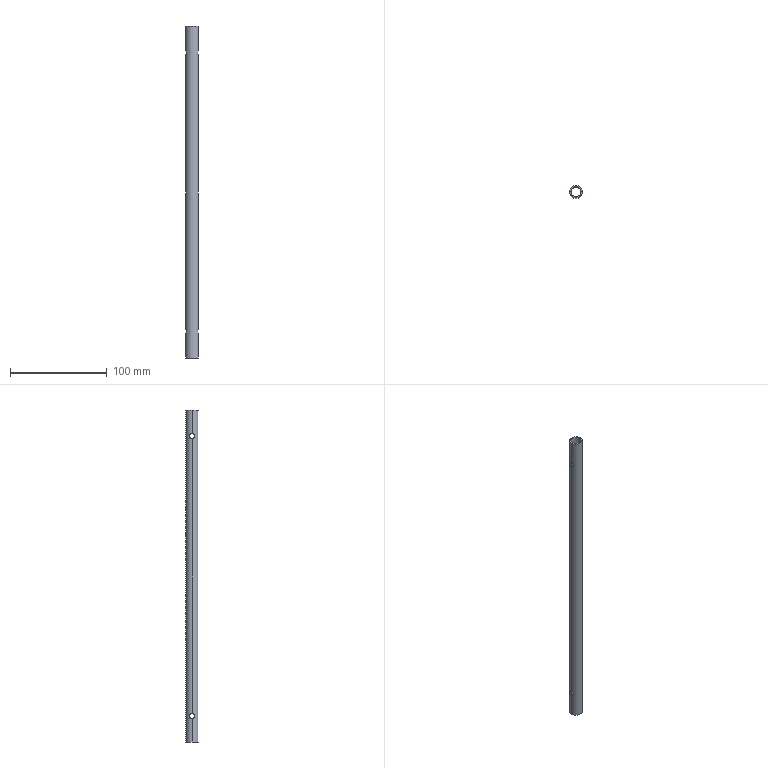Part | SolidWorks | features BaseBody 1 | 1 solid | 14 faces | box 13 x 13 x 343 mm | volume 15154 mm3 | cylinder 12 | plane 2 | commonest cylinder face diameters 5.2 x8 10.6 x2 13 x2
STEP:
#1=CARTESIAN_POINT('',(-6.5,0.,343.));
#2=VERTEX_POINT('',#1);
#3=CARTESIAN_POINT('',(6.5,0.,343.));
#4=VERTEX_POINT('',#3);
#5=CARTESIAN_POINT('',(0.,0.,343.));
#6=DIRECTION('',(0.,0.,-1.));
#7=DIRECTION('',(-1.,0.,0.));
#8=AXIS2_PLACEMENT_3D('',#5,#6,#7);
#9=CIRCLE('',#8,6.5);
#10=EDGE_CURVE('',#2,#4,#9,.T.);
#11=ORIENTED_EDGE('',*,*,#10,.T.);
#12=CARTESIAN_POINT('',(6.5,0.,318.6));
#13=VERTEX_POINT('',#12);
#14=CARTESIAN_POINT('',(6.5,0.,343.));
#15=DIRECTION('',(0.,0.,-1.));
#16=VECTOR('',#15,1000.);
#17=LINE('',#14,#16);
#18=EDGE_CURVE('',#4,#13,#17,.T.);
#19=ORIENTED_EDGE('',*,*,#18,.T.);
#20=CARTESIAN_POINT('',(6.5,0.,313.4));
#21=VERTEX_POINT('',#20);
#22=CARTESIAN_POINT('',(6.5,0.,318.6));
#23=CARTESIAN_POINT('',(6.5,0.1737,318.6));
#24=CARTESIAN_POINT('',(6.493,0.3441,318.583));
#25=CARTESIAN_POINT('',(6.467,0.6788,318.516));
#26=CARTESIAN_POINT('',(6.447,0.8449,318.465));
#27=CARTESIAN_POINT('',(6.398,1.159,318.334));
#28=CARTESIAN_POINT('',(6.369,1.308,318.254));
#29=CARTESIAN_POINT('',(6.304,1.589,318.065));
#30=CARTESIAN_POINT('',(6.269,1.72,317.957));
#31=CARTESIAN_POINT('',(6.165,2.076,317.601));
#32=CARTESIAN_POINT('',(6.093,2.269,317.314));
#33=CARTESIAN_POINT('',(6.015,2.464,316.847));
#34=CARTESIAN_POINT('',(5.994,2.515,316.681));
#35=CARTESIAN_POINT('',(5.965,2.583,316.345));
#36=CARTESIAN_POINT('',(5.957,2.6,316.175));
#37=CARTESIAN_POINT('',(5.957,2.6,315.832));
#38=CARTESIAN_POINT('',(5.965,2.583,315.658));
#39=CARTESIAN_POINT('',(5.993,2.516,315.323));
#40=CARTESIAN_POINT('',(6.014,2.466,315.159));
#41=CARTESIAN_POINT('',(6.067,2.335,314.843));
#42=CARTESIAN_POINT('',(6.097,2.254,314.694));
#43=CARTESIAN_POINT('',(6.163,2.067,314.414));
#44=CARTESIAN_POINT('',(6.199,1.959,314.282));
#45=CARTESIAN_POINT('',(6.269,1.721,314.044));
#46=CARTESIAN_POINT('',(6.304,1.592,313.937));
#47=CARTESIAN_POINT('',(6.368,1.311,313.748));
#48=CARTESIAN_POINT('',(6.398,1.16,313.667));
#49=CARTESIAN_POINT('',(6.471,0.6911,313.471));
#50=CARTESIAN_POINT('',(6.5,0.3472,313.4));
#51=CARTESIAN_POINT('',(6.5,0.,313.4));
#52=B_SPLINE_CURVE_WITH_KNOTS('',3,(#22,#23,#24,#25,#26,#27,#28,#29,#30,#31,#32,#33,#34,#35,#36,#37,#38,#39,#40,#41,#42,#43,#44,#45,#46,#47,#48,#49,#50,#51),.UNSPECIFIED.,.F.,.F.,(4,2,2,2,2,2,2,2,2,2,2,2,2,2,4),(0.008212,0.008725,0.009238,0.009751,0.01026,0.01129,0.0118,0.01232,0.01283,0.01334,0.01386,0.01437,0.01488,0.0154,0.01642),.UNSPECIFIED.);
#53=EDGE_CURVE('',#13,#21,#52,.T.);
#54=ORIENTED_EDGE('',*,*,#53,.T.);
#55=CARTESIAN_POINT('',(6.5,0.,29.6));
#56=VERTEX_POINT('',#55);
#57=CARTESIAN_POINT('',(6.5,0.,343.));
#58=DIRECTION('',(0.,0.,-1.));
#59=VECTOR('',#58,1000.);
#60=LINE('',#57,#59);
#61=EDGE_CURVE('',#21,#56,#60,.T.);
#62=ORIENTED_EDGE('',*,*,#61,.T.);
#63=CARTESIAN_POINT('',(6.5,0.,24.4));
#64=VERTEX_POINT('',#63);
#65=CARTESIAN_POINT('',(6.5,0.,29.6));
#66=CARTESIAN_POINT('',(6.5,0.1737,29.6));
#67=CARTESIAN_POINT('',(6.493,0.3441,29.583));
#68=CARTESIAN_POINT('',(6.467,0.6788,29.516));
#69=CARTESIAN_POINT('',(6.447,0.8449,29.465));
#70=CARTESIAN_POINT('',(6.398,1.159,29.334));
#71=CARTESIAN_POINT('',(6.369,1.308,29.254));
#72=CARTESIAN_POINT('',(6.304,1.589,29.065));
#73=CARTESIAN_POINT('',(6.269,1.72,28.957));
#74=CARTESIAN_POINT('',(6.165,2.076,28.601));
#75=CARTESIAN_POINT('',(6.093,2.269,28.314));
#76=CARTESIAN_POINT('',(6.015,2.464,27.847));
#77=CARTESIAN_POINT('',(5.994,2.515,27.681));
#78=CARTESIAN_POINT('',(5.965,2.583,27.345));
#79=CARTESIAN_POINT('',(5.957,2.6,27.175));
#80=CARTESIAN_POINT('',(5.957,2.6,26.832));
#81=CARTESIAN_POINT('',(5.965,2.583,26.658));
#82=CARTESIAN_POINT('',(5.993,2.516,26.323));
#83=CARTESIAN_POINT('',(6.014,2.466,26.159));
#84=CARTESIAN_POINT('',(6.067,2.335,25.843));
#85=CARTESIAN_POINT('',(6.097,2.254,25.694));
#86=CARTESIAN_POINT('',(6.163,2.067,25.414));
#87=CARTESIAN_POINT('',(6.199,1.959,25.282));
#88=CARTESIAN_POINT('',(6.269,1.721,25.044));
#89=CARTESIAN_POINT('',(6.304,1.592,24.937));
#90=CARTESIAN_POINT('',(6.368,1.311,24.748));
#91=CARTESIAN_POINT('',(6.398,1.16,24.667));
#92=CARTESIAN_POINT('',(6.471,0.6911,24.471));
#93=CARTESIAN_POINT('',(6.5,0.3472,24.4));
#94=CARTESIAN_POINT('',(6.5,0.,24.4));
#95=B_SPLINE_CURVE_WITH_KNOTS('',3,(#65,#66,#67,#68,#69,#70,#71,#72,#73,#74,#75,#76,#77,#78,#79,#80,#81,#82,#83,#84,#85,#86,#87,#88,#89,#90,#91,#92,#93,#94),.UNSPECIFIED.,.F.,.F.,(4,2,2,2,2,2,2,2,2,2,2,2,2,2,4),(0.008212,0.008725,0.009238,0.009751,0.01026,0.01129,0.0118,0.01232,0.01283,0.01334,0.01386,0.01437,0.01488,0.0154,0.01642),.UNSPECIFIED.);
#96=EDGE_CURVE('',#56,#64,#95,.T.);
#97=ORIENTED_EDGE('',*,*,#96,.T.);
#98=CARTESIAN_POINT('',(6.5,0.,0.));
#99=VERTEX_POINT('',#98);
#100=CARTESIAN_POINT('',(6.5,0.,343.));
#101=DIRECTION('',(0.,0.,-1.));
#102=VECTOR('',#101,1000.);
#103=LINE('',#100,#102);
#104=EDGE_CURVE('',#64,#99,#103,.T.);
#105=ORIENTED_EDGE('',*,*,#104,.T.);
#106=CARTESIAN_POINT('',(-6.5,0.,0.));
#107=VERTEX_POINT('',#106);
#108=CARTESIAN_POINT('',(0.,0.,0.));
#109=DIRECTION('',(0.,0.,1.));
#110=DIRECTION('',(-1.,0.,0.));
#111=AXIS2_PLACEMENT_3D('',#108,#109,#110);
#112=CIRCLE('',#111,6.5);
#113=EDGE_CURVE('',#99,#107,#112,.T.);
#114=ORIENTED_EDGE('',*,*,#113,.T.);
#115=CARTESIAN_POINT('',(-6.5,0.,24.4));
#116=VERTEX_POINT('',#115);
#117=CARTESIAN_POINT('',(-6.5,0.,343.));
#118=DIRECTION('',(0.,0.,-1.));
#119=VECTOR('',#118,1000.);
#120=LINE('',#117,#119);
#121=EDGE_CURVE('',#116,#107,#120,.T.);
#122=ORIENTED_EDGE('',*,*,#121,.F.);
#123=CARTESIAN_POINT('',(-6.5,0.,29.6));
#124=VERTEX_POINT('',#123);
#125=CARTESIAN_POINT('',(-6.5,0.,24.4));
#126=CARTESIAN_POINT('',(-6.5,0.1737,24.4));
#127=CARTESIAN_POINT('',(-6.493,0.3441,24.417));
#128=CARTESIAN_POINT('',(-6.467,0.6788,24.484));
#129=CARTESIAN_POINT('',(-6.447,0.8449,24.535));
#130=CARTESIAN_POINT('',(-6.398,1.159,24.666));
#131=CARTESIAN_POINT('',(-6.369,1.308,24.746));
#132=CARTESIAN_POINT('',(-6.304,1.589,24.935));
#133=CARTESIAN_POINT('',(-6.269,1.72,25.043));
#134=CARTESIAN_POINT('',(-6.165,2.076,25.399));
#135=CARTESIAN_POINT('',(-6.093,2.269,25.686));
#136=CARTESIAN_POINT('',(-6.015,2.464,26.153));
#137=CARTESIAN_POINT('',(-5.994,2.515,26.319));
#138=CARTESIAN_POINT('',(-5.965,2.583,26.655));
#139=CARTESIAN_POINT('',(-5.957,2.6,26.825));
#140=CARTESIAN_POINT('',(-5.957,2.6,27.168));
#141=CARTESIAN_POINT('',(-5.965,2.583,27.342));
#142=CARTESIAN_POINT('',(-5.993,2.516,27.677));
#143=CARTESIAN_POINT('',(-6.014,2.466,27.841));
#144=CARTESIAN_POINT('',(-6.067,2.335,28.157));
#145=CARTESIAN_POINT('',(-6.097,2.254,28.306));
#146=CARTESIAN_POINT('',(-6.163,2.067,28.586));
#147=CARTESIAN_POINT('',(-6.199,1.959,28.718));
#148=CARTESIAN_POINT('',(-6.269,1.721,28.956));
#149=CARTESIAN_POINT('',(-6.304,1.592,29.063));
#150=CARTESIAN_POINT('',(-6.368,1.311,29.252));
#151=CARTESIAN_POINT('',(-6.398,1.16,29.333));
#152=CARTESIAN_POINT('',(-6.471,0.6911,29.529));
#153=CARTESIAN_POINT('',(-6.5,0.3472,29.6));
#154=CARTESIAN_POINT('',(-6.5,0.,29.6));
#155=B_SPLINE_CURVE_WITH_KNOTS('',3,(#125,#126,#127,#128,#129,#130,#131,#132,#133,#134,#135,#136,#137,#138,#139,#140,#141,#142,#143,#144,#145,#146,#147,#148,#149,#150,#151,#152,#153,#154),.UNSPECIFIED.,.F.,.F.,(4,2,2,2,2,2,2,2,2,2,2,2,2,2,4),(0.008212,0.008725,0.009238,0.009751,0.01026,0.01129,0.0118,0.01232,0.01283,0.01334,0.01386,0.01437,0.01488,0.0154,0.01642),.UNSPECIFIED.);
#156=EDGE_CURVE('',#116,#124,#155,.T.);
#157=ORIENTED_EDGE('',*,*,#156,.T.);
#158=CARTESIAN_POINT('',(-6.5,0.,313.4));
#159=VERTEX_POINT('',#158);
#160=CARTESIAN_POINT('',(-6.5,0.,343.));
#161=DIRECTION('',(0.,0.,-1.));
#162=VECTOR('',#161,1000.);
#163=LINE('',#160,#162);
#164=EDGE_CURVE('',#159,#124,#163,.T.);
#165=ORIENTED_EDGE('',*,*,#164,.F.);
#166=CARTESIAN_POINT('',(-6.5,0.,318.6));
#167=VERTEX_POINT('',#166);
#168=CARTESIAN_POINT('',(-6.5,0.,313.4));
#169=CARTESIAN_POINT('',(-6.5,0.1737,313.4));
#170=CARTESIAN_POINT('',(-6.493,0.3441,313.417));
#171=CARTESIAN_POINT('',(-6.467,0.6788,313.484));
#172=CARTESIAN_POINT('',(-6.447,0.8449,313.535));
#173=CARTESIAN_POINT('',(-6.398,1.159,313.666));
#174=CARTESIAN_POINT('',(-6.369,1.308,313.746));
#175=CARTESIAN_POINT('',(-6.304,1.589,313.935));
#176=CARTESIAN_POINT('',(-6.269,1.72,314.043));
#177=CARTESIAN_POINT('',(-6.165,2.076,314.399));
#178=CARTESIAN_POINT('',(-6.093,2.269,314.686));
#179=CARTESIAN_POINT('',(-6.015,2.464,315.153));
#180=CARTESIAN_POINT('',(-5.994,2.515,315.319));
#181=CARTESIAN_POINT('',(-5.965,2.583,315.655));
#182=CARTESIAN_POINT('',(-5.957,2.6,315.825));
#183=CARTESIAN_POINT('',(-5.957,2.6,316.168));
#184=CARTESIAN_POINT('',(-5.965,2.583,316.342));
#185=CARTESIAN_POINT('',(-5.993,2.516,316.677));
#186=CARTESIAN_POINT('',(-6.014,2.466,316.841));
#187=CARTESIAN_POINT('',(-6.067,2.335,317.157));
#188=CARTESIAN_POINT('',(-6.097,2.254,317.306));
#189=CARTESIAN_POINT('',(-6.163,2.067,317.586));
#190=CARTESIAN_POINT('',(-6.199,1.959,317.718));
#191=CARTESIAN_POINT('',(-6.269,1.721,317.956));
#192=CARTESIAN_POINT('',(-6.304,1.592,318.063));
#193=CARTESIAN_POINT('',(-6.368,1.311,318.252));
#194=CARTESIAN_POINT('',(-6.398,1.16,318.333));
#195=CARTESIAN_POINT('',(-6.471,0.6911,318.529));
#196=CARTESIAN_POINT('',(-6.5,0.3472,318.6));
#197=CARTESIAN_POINT('',(-6.5,0.,318.6));
#198=B_SPLINE_CURVE_WITH_KNOTS('',3,(#168,#169,#170,#171,#172,#173,#174,#175,#176,#177,#178,#179,#180,#181,#182,#183,#184,#185,#186,#187,#188,#189,#190,#191,#192,#193,#194,#195,#196,#197),.UNSPECIFIED.,.F.,.F.,(4,2,2,2,2,2,2,2,2,2,2,2,2,2,4),(0.008212,0.008725,0.009238,0.009751,0.01026,0.01129,0.0118,0.01232,0.01283,0.01334,0.01386,0.01437,0.01488,0.0154,0.01642),.UNSPECIFIED.);
#199=EDGE_CURVE('',#159,#167,#198,.T.);
#200=ORIENTED_EDGE('',*,*,#199,.T.);
#201=CARTESIAN_POINT('',(-6.5,0.,343.));
#202=DIRECTION('',(0.,0.,-1.));
#203=VECTOR('',#202,1000.);
#204=LINE('',#201,#203);
#205=EDGE_CURVE('',#2,#167,#204,.T.);
#206=ORIENTED_EDGE('',*,*,#205,.F.);
#207=EDGE_LOOP('',(#11,#19,#54,#62,#97,#105,#114,#122,#157,#165,#200,#206));
#208=FACE_OUTER_BOUND('',#207,.T.);
#209=CARTESIAN_POINT('',(0.,0.,343.));
#210=DIRECTION('',(0.,0.,-1.));
#211=DIRECTION('',(-1.,0.,0.));
#212=AXIS2_PLACEMENT_3D('',#209,#210,#211);
#213=CYLINDRICAL_SURFACE('',#212,6.5);
#214=ADVANCED_FACE('',(#208),#213,.T.);
#215=CARTESIAN_POINT('',(5.3,0.,318.6));
#216=VERTEX_POINT('',#215);
#217=CARTESIAN_POINT('',(5.3,0.,313.4));
#218=VERTEX_POINT('',#217);
#219=CARTESIAN_POINT('',(5.3,0.,318.6));
#220=CARTESIAN_POINT('',(5.3,-0.1748,318.6));
#221=CARTESIAN_POINT('',(5.291,-0.3461,318.583));
#222=CARTESIAN_POINT('',(5.259,-0.6823,318.515));
#223=CARTESIAN_POINT('',(5.234,-0.8489,318.463));
#224=CARTESIAN_POINT('',(5.173,-1.163,318.332));
#225=CARTESIAN_POINT('',(5.137,-1.311,318.252));
#226=CARTESIAN_POINT('',(5.057,-1.592,318.063));
#227=CARTESIAN_POINT('',(5.014,-1.722,317.955));
#228=CARTESIAN_POINT('',(4.927,-1.958,317.719));
#229=CARTESIAN_POINT('',(4.882,-2.065,317.589));
#230=CARTESIAN_POINT('',(4.799,-2.253,317.309));
#231=CARTESIAN_POINT('',(4.76,-2.332,317.162));
#232=CARTESIAN_POINT('',(4.694,-2.463,316.85));
#233=CARTESIAN_POINT('',(4.666,-2.514,316.684));
#234=CARTESIAN_POINT('',(4.628,-2.582,316.348));
#235=CARTESIAN_POINT('',(4.619,-2.6,316.177));
#236=CARTESIAN_POINT('',(4.618,-2.6,315.832));
#237=CARTESIAN_POINT('',(4.628,-2.583,315.657));
#238=CARTESIAN_POINT('',(4.665,-2.515,315.32));
#239=CARTESIAN_POINT('',(4.693,-2.465,315.155));
#240=CARTESIAN_POINT('',(4.759,-2.333,314.84));
#241=CARTESIAN_POINT('',(4.798,-2.253,314.692));
#242=CARTESIAN_POINT('',(4.882,-2.066,314.413));
#243=CARTESIAN_POINT('',(4.926,-1.959,314.282));
#244=CARTESIAN_POINT('',(5.014,-1.723,314.046));
#245=CARTESIAN_POINT('',(5.057,-1.594,313.939));
#246=CARTESIAN_POINT('',(5.137,-1.313,313.749));
#247=CARTESIAN_POINT('',(5.173,-1.164,313.669));
#248=CARTESIAN_POINT('',(5.233,-0.8519,313.538));
#249=CARTESIAN_POINT('',(5.258,-0.6876,313.487));
#250=CARTESIAN_POINT('',(5.291,-0.3474,313.417));
#251=CARTESIAN_POINT('',(5.3,-0.1749,313.4));
#252=CARTESIAN_POINT('',(5.3,0.,313.4));
#253=B_SPLINE_CURVE_WITH_KNOTS('',3,(#219,#220,#221,#222,#223,#224,#225,#226,#227,#228,#229,#230,#231,#232,#233,#234,#235,#236,#237,#238,#239,#240,#241,#242,#243,#244,#245,#246,#247,#248,#249,#250,#251,#252),.UNSPECIFIED.,.F.,.F.,(4,2,2,2,2,2,2,2,2,2,2,2,2,2,2,2,4),(0.,0.0005163,0.001033,0.001549,0.002065,0.002581,0.003098,0.003614,0.00413,0.004646,0.005163,0.005679,0.006195,0.006712,0.007228,0.007744,0.00826),.UNSPECIFIED.);
#254=EDGE_CURVE('',#216,#218,#253,.T.);
#255=ORIENTED_EDGE('',*,*,#254,.F.);
#256=CARTESIAN_POINT('',(-6.5,0.,318.6));
#257=DIRECTION('',(1.,0.,0.));
#258=VECTOR('',#257,1000.);
#259=LINE('',#256,#258);
#260=EDGE_CURVE('',#216,#13,#259,.T.);
#261=ORIENTED_EDGE('',*,*,#260,.T.);
#262=CARTESIAN_POINT('',(6.5,0.,313.4));
#263=CARTESIAN_POINT('',(6.5,-0.1737,313.4));
#264=CARTESIAN_POINT('',(6.493,-0.3441,313.417));
#265=CARTESIAN_POINT('',(6.467,-0.6788,313.484));
#266=CARTESIAN_POINT('',(6.447,-0.8449,313.535));
#267=CARTESIAN_POINT('',(6.398,-1.159,313.666));
#268=CARTESIAN_POINT('',(6.369,-1.308,313.746));
#269=CARTESIAN_POINT('',(6.304,-1.589,313.935));
#270=CARTESIAN_POINT('',(6.269,-1.72,314.043));
#271=CARTESIAN_POINT('',(6.165,-2.076,314.399));
#272=CARTESIAN_POINT('',(6.093,-2.269,314.686));
#273=CARTESIAN_POINT('',(6.015,-2.464,315.153));
#274=CARTESIAN_POINT('',(5.994,-2.515,315.319));
#275=CARTESIAN_POINT('',(5.965,-2.583,315.655));
#276=CARTESIAN_POINT('',(5.957,-2.6,315.825));
#277=CARTESIAN_POINT('',(5.957,-2.6,316.168));
#278=CARTESIAN_POINT('',(5.965,-2.583,316.342));
#279=CARTESIAN_POINT('',(5.993,-2.516,316.677));
#280=CARTESIAN_POINT('',(6.014,-2.466,316.841));
#281=CARTESIAN_POINT('',(6.067,-2.335,317.157));
#282=CARTESIAN_POINT('',(6.097,-2.254,317.306));
#283=CARTESIAN_POINT('',(6.163,-2.067,317.586));
#284=CARTESIAN_POINT('',(6.199,-1.959,317.718));
#285=CARTESIAN_POINT('',(6.269,-1.721,317.956));
#286=CARTESIAN_POINT('',(6.304,-1.592,318.063));
#287=CARTESIAN_POINT('',(6.368,-1.311,318.252));
#288=CARTESIAN_POINT('',(6.398,-1.16,318.333));
#289=CARTESIAN_POINT('',(6.471,-0.6911,318.529));
#290=CARTESIAN_POINT('',(6.5,-0.3475,318.6));
#291=CARTESIAN_POINT('',(6.5,0.,318.6));
#292=B_SPLINE_CURVE_WITH_KNOTS('',3,(#262,#263,#264,#265,#266,#267,#268,#269,#270,#271,#272,#273,#274,#275,#276,#277,#278,#279,#280,#281,#282,#283,#284,#285,#286,#287,#288,#289,#290,#291),.UNSPECIFIED.,.F.,.F.,(4,2,2,2,2,2,2,2,2,2,2,2,2,2,4),(0.,0.0005133,0.001027,0.00154,0.002053,0.00308,0.003593,0.004106,0.004619,0.005133,0.005646,0.006159,0.006672,0.007186,0.008212),.UNSPECIFIED.);
#293=EDGE_CURVE('',#21,#13,#292,.T.);
#294=ORIENTED_EDGE('',*,*,#293,.F.);
#295=CARTESIAN_POINT('',(-6.5,0.,313.4));
#296=DIRECTION('',(1.,0.,0.));
#297=VECTOR('',#296,1000.);
#298=LINE('',#295,#297);
#299=EDGE_CURVE('',#218,#21,#298,.T.);
#300=ORIENTED_EDGE('',*,*,#299,.F.);
#301=EDGE_LOOP('',(#255,#261,#294,#300));
#302=FACE_OUTER_BOUND('',#301,.T.);
#303=CARTESIAN_POINT('',(-6.5,0.,316.));
#304=DIRECTION('',(1.,0.,0.));
#305=DIRECTION('',(0.,0.,-1.));
#306=AXIS2_PLACEMENT_3D('',#303,#304,#305);
#307=CYLINDRICAL_SURFACE('',#306,2.6);
#308=ADVANCED_FACE('',(#302),#307,.F.);
#309=CARTESIAN_POINT('',(5.3,0.,29.6));
#310=VERTEX_POINT('',#309);
#311=CARTESIAN_POINT('',(5.3,0.,24.4));
#312=VERTEX_POINT('',#311);
#313=CARTESIAN_POINT('',(5.3,0.,29.6));
#314=CARTESIAN_POINT('',(5.3,-0.1748,29.6));
#315=CARTESIAN_POINT('',(5.291,-0.3461,29.583));
#316=CARTESIAN_POINT('',(5.259,-0.6823,29.515));
#317=CARTESIAN_POINT('',(5.234,-0.8489,29.463));
#318=CARTESIAN_POINT('',(5.173,-1.163,29.332));
#319=CARTESIAN_POINT('',(5.137,-1.311,29.252));
#320=CARTESIAN_POINT('',(5.057,-1.592,29.063));
#321=CARTESIAN_POINT('',(5.014,-1.722,28.955));
#322=CARTESIAN_POINT('',(4.927,-1.958,28.719));
#323=CARTESIAN_POINT('',(4.882,-2.065,28.589));
#324=CARTESIAN_POINT('',(4.799,-2.253,28.309));
#325=CARTESIAN_POINT('',(4.76,-2.332,28.162));
#326=CARTESIAN_POINT('',(4.694,-2.463,27.85));
#327=CARTESIAN_POINT('',(4.666,-2.514,27.684));
#328=CARTESIAN_POINT('',(4.628,-2.582,27.348));
#329=CARTESIAN_POINT('',(4.619,-2.6,27.177));
#330=CARTESIAN_POINT('',(4.618,-2.6,26.832));
#331=CARTESIAN_POINT('',(4.628,-2.583,26.657));
#332=CARTESIAN_POINT('',(4.665,-2.515,26.32));
#333=CARTESIAN_POINT('',(4.693,-2.465,26.155));
#334=CARTESIAN_POINT('',(4.759,-2.333,25.84));
#335=CARTESIAN_POINT('',(4.798,-2.253,25.692));
#336=CARTESIAN_POINT('',(4.882,-2.066,25.413));
#337=CARTESIAN_POINT('',(4.926,-1.959,25.282));
#338=CARTESIAN_POINT('',(5.014,-1.723,25.046));
#339=CARTESIAN_POINT('',(5.057,-1.594,24.939));
#340=CARTESIAN_POINT('',(5.137,-1.313,24.749));
#341=CARTESIAN_POINT('',(5.173,-1.164,24.669));
#342=CARTESIAN_POINT('',(5.233,-0.8519,24.538));
#343=CARTESIAN_POINT('',(5.258,-0.6876,24.487));
#344=CARTESIAN_POINT('',(5.291,-0.3474,24.417));
#345=CARTESIAN_POINT('',(5.3,-0.1749,24.4));
#346=CARTESIAN_POINT('',(5.3,0.,24.4));
#347=B_SPLINE_CURVE_WITH_KNOTS('',3,(#313,#314,#315,#316,#317,#318,#319,#320,#321,#322,#323,#324,#325,#326,#327,#328,#329,#330,#331,#332,#333,#334,#335,#336,#337,#338,#339,#340,#341,#342,#343,#344,#345,#346),.UNSPECIFIED.,.F.,.F.,(4,2,2,2,2,2,2,2,2,2,2,2,2,2,2,2,4),(0.,0.0005163,0.001033,0.001549,0.002065,0.002581,0.003098,0.003614,0.00413,0.004646,0.005163,0.005679,0.006195,0.006712,0.007228,0.007744,0.00826),.UNSPECIFIED.);
#348=EDGE_CURVE('',#310,#312,#347,.T.);
#349=ORIENTED_EDGE('',*,*,#348,.F.);
#350=CARTESIAN_POINT('',(-6.5,0.,29.6));
#351=DIRECTION('',(1.,0.,0.));
#352=VECTOR('',#351,1000.);
#353=LINE('',#350,#352);
#354=EDGE_CURVE('',#310,#56,#353,.T.);
#355=ORIENTED_EDGE('',*,*,#354,.T.);
#356=CARTESIAN_POINT('',(6.5,0.,24.4));
#357=CARTESIAN_POINT('',(6.5,-0.1737,24.4));
#358=CARTESIAN_POINT('',(6.493,-0.3441,24.417));
#359=CARTESIAN_POINT('',(6.467,-0.6788,24.484));
#360=CARTESIAN_POINT('',(6.447,-0.8449,24.535));
#361=CARTESIAN_POINT('',(6.398,-1.159,24.666));
#362=CARTESIAN_POINT('',(6.369,-1.308,24.746));
#363=CARTESIAN_POINT('',(6.304,-1.589,24.935));
#364=CARTESIAN_POINT('',(6.269,-1.72,25.043));
#365=CARTESIAN_POINT('',(6.165,-2.076,25.399));
#366=CARTESIAN_POINT('',(6.093,-2.269,25.686));
#367=CARTESIAN_POINT('',(6.015,-2.464,26.153));
#368=CARTESIAN_POINT('',(5.994,-2.515,26.319));
#369=CARTESIAN_POINT('',(5.965,-2.583,26.655));
#370=CARTESIAN_POINT('',(5.957,-2.6,26.825));
#371=CARTESIAN_POINT('',(5.957,-2.6,27.168));
#372=CARTESIAN_POINT('',(5.965,-2.583,27.342));
#373=CARTESIAN_POINT('',(5.993,-2.516,27.677));
#374=CARTESIAN_POINT('',(6.014,-2.466,27.841));
#375=CARTESIAN_POINT('',(6.067,-2.335,28.157));
#376=CARTESIAN_POINT('',(6.097,-2.254,28.306));
#377=CARTESIAN_POINT('',(6.163,-2.067,28.586));
#378=CARTESIAN_POINT('',(6.199,-1.959,28.718));
#379=CARTESIAN_POINT('',(6.269,-1.721,28.956));
#380=CARTESIAN_POINT('',(6.304,-1.592,29.063));
#381=CARTESIAN_POINT('',(6.368,-1.311,29.252));
#382=CARTESIAN_POINT('',(6.398,-1.16,29.333));
#383=CARTESIAN_POINT('',(6.471,-0.6911,29.529));
#384=CARTESIAN_POINT('',(6.5,-0.3475,29.6));
#385=CARTESIAN_POINT('',(6.5,0.,29.6));
#386=B_SPLINE_CURVE_WITH_KNOTS('',3,(#356,#357,#358,#359,#360,#361,#362,#363,#364,#365,#366,#367,#368,#369,#370,#371,#372,#373,#374,#375,#376,#377,#378,#379,#380,#381,#382,#383,#384,#385),.UNSPECIFIED.,.F.,.F.,(4,2,2,2,2,2,2,2,2,2,2,2,2,2,4),(0.,0.0005133,0.001027,0.00154,0.002053,0.00308,0.003593,0.004106,0.004619,0.005133,0.005646,0.006159,0.006672,0.007186,0.008212),.UNSPECIFIED.);
#387=EDGE_CURVE('',#64,#56,#386,.T.);
#388=ORIENTED_EDGE('',*,*,#387,.F.);
#389=CARTESIAN_POINT('',(-6.5,0.,24.4));
#390=DIRECTION('',(1.,0.,0.));
#391=VECTOR('',#390,1000.);
#392=LINE('',#389,#391);
#393=EDGE_CURVE('',#312,#64,#392,.T.);
#394=ORIENTED_EDGE('',*,*,#393,.F.);
#395=EDGE_LOOP('',(#349,#355,#388,#394));
#396=FACE_OUTER_BOUND('',#395,.T.);
#397=CARTESIAN_POINT('',(-6.5,0.,27.));
#398=DIRECTION('',(1.,0.,0.));
#399=DIRECTION('',(0.,0.,-1.));
#400=AXIS2_PLACEMENT_3D('',#397,#398,#399);
#401=CYLINDRICAL_SURFACE('',#400,2.6);
#402=ADVANCED_FACE('',(#396),#401,.F.);
#403=CARTESIAN_POINT('',(-6.5,0.,29.6));
#404=CARTESIAN_POINT('',(-6.5,-0.1737,29.6));
#405=CARTESIAN_POINT('',(-6.493,-0.3441,29.583));
#406=CARTESIAN_POINT('',(-6.467,-0.6788,29.516));
#407=CARTESIAN_POINT('',(-6.447,-0.8449,29.465));
#408=CARTESIAN_POINT('',(-6.398,-1.159,29.334));
#409=CARTESIAN_POINT('',(-6.369,-1.308,29.254));
#410=CARTESIAN_POINT('',(-6.304,-1.589,29.065));
#411=CARTESIAN_POINT('',(-6.269,-1.72,28.957));
#412=CARTESIAN_POINT('',(-6.165,-2.076,28.601));
#413=CARTESIAN_POINT('',(-6.093,-2.269,28.314));
#414=CARTESIAN_POINT('',(-6.015,-2.464,27.847));
#415=CARTESIAN_POINT('',(-5.994,-2.515,27.681));
#416=CARTESIAN_POINT('',(-5.965,-2.583,27.345));
#417=CARTESIAN_POINT('',(-5.957,-2.6,27.175));
#418=CARTESIAN_POINT('',(-5.957,-2.6,26.832));
#419=CARTESIAN_POINT('',(-5.965,-2.583,26.658));
#420=CARTESIAN_POINT('',(-5.993,-2.516,26.323));
#421=CARTESIAN_POINT('',(-6.014,-2.466,26.159));
#422=CARTESIAN_POINT('',(-6.067,-2.335,25.843));
#423=CARTESIAN_POINT('',(-6.097,-2.254,25.694));
#424=CARTESIAN_POINT('',(-6.163,-2.067,25.414));
#425=CARTESIAN_POINT('',(-6.199,-1.959,25.282));
#426=CARTESIAN_POINT('',(-6.269,-1.721,25.044));
#427=CARTESIAN_POINT('',(-6.304,-1.592,24.937));
#428=CARTESIAN_POINT('',(-6.368,-1.311,24.748));
#429=CARTESIAN_POINT('',(-6.398,-1.16,24.667));
#430=CARTESIAN_POINT('',(-6.471,-0.6911,24.471));
#431=CARTESIAN_POINT('',(-6.5,-0.3475,24.4));
#432=CARTESIAN_POINT('',(-6.5,0.,24.4));
#433=B_SPLINE_CURVE_WITH_KNOTS('',3,(#403,#404,#405,#406,#407,#408,#409,#410,#411,#412,#413,#414,#415,#416,#417,#418,#419,#420,#421,#422,#423,#424,#425,#426,#427,#428,#429,#430,#431,#432),.UNSPECIFIED.,.F.,.F.,(4,2,2,2,2,2,2,2,2,2,2,2,2,2,4),(0.,0.0005133,0.001027,0.00154,0.002053,0.00308,0.003593,0.004106,0.004619,0.005133,0.005646,0.006159,0.006672,0.007186,0.008212),.UNSPECIFIED.);
#434=EDGE_CURVE('',#124,#116,#433,.T.);
#435=ORIENTED_EDGE('',*,*,#434,.F.);
#436=CARTESIAN_POINT('',(-5.3,0.,29.6));
#437=VERTEX_POINT('',#436);
#438=CARTESIAN_POINT('',(-6.5,0.,29.6));
#439=DIRECTION('',(1.,0.,0.));
#440=VECTOR('',#439,1000.);
#441=LINE('',#438,#440);
#442=EDGE_CURVE('',#124,#437,#441,.T.);
#443=ORIENTED_EDGE('',*,*,#442,.T.);
#444=CARTESIAN_POINT('',(-5.3,0.,24.4));
#445=VERTEX_POINT('',#444);
#446=CARTESIAN_POINT('',(-5.3,0.,24.4));
#447=CARTESIAN_POINT('',(-5.3,-0.1748,24.4));
#448=CARTESIAN_POINT('',(-5.291,-0.3461,24.417));
#449=CARTESIAN_POINT('',(-5.259,-0.6823,24.485));
#450=CARTESIAN_POINT('',(-5.234,-0.8489,24.537));
#451=CARTESIAN_POINT('',(-5.173,-1.163,24.668));
#452=CARTESIAN_POINT('',(-5.137,-1.311,24.748));
#453=CARTESIAN_POINT('',(-5.057,-1.592,24.937));
#454=CARTESIAN_POINT('',(-5.014,-1.722,25.045));
#455=CARTESIAN_POINT('',(-4.927,-1.958,25.281));
#456=CARTESIAN_POINT('',(-4.882,-2.065,25.411));
#457=CARTESIAN_POINT('',(-4.799,-2.253,25.691));
#458=CARTESIAN_POINT('',(-4.76,-2.332,25.838));
#459=CARTESIAN_POINT('',(-4.694,-2.463,26.15));
#460=CARTESIAN_POINT('',(-4.666,-2.514,26.316));
#461=CARTESIAN_POINT('',(-4.628,-2.582,26.652));
#462=CARTESIAN_POINT('',(-4.619,-2.6,26.823));
#463=CARTESIAN_POINT('',(-4.618,-2.6,27.168));
#464=CARTESIAN_POINT('',(-4.628,-2.583,27.343));
#465=CARTESIAN_POINT('',(-4.665,-2.515,27.68));
#466=CARTESIAN_POINT('',(-4.693,-2.465,27.845));
#467=CARTESIAN_POINT('',(-4.759,-2.333,28.16));
#468=CARTESIAN_POINT('',(-4.798,-2.253,28.308));
#469=CARTESIAN_POINT('',(-4.882,-2.066,28.587));
#470=CARTESIAN_POINT('',(-4.926,-1.959,28.718));
#471=CARTESIAN_POINT('',(-5.014,-1.723,28.954));
#472=CARTESIAN_POINT('',(-5.057,-1.594,29.061));
#473=CARTESIAN_POINT('',(-5.137,-1.313,29.251));
#474=CARTESIAN_POINT('',(-5.173,-1.164,29.331));
#475=CARTESIAN_POINT('',(-5.233,-0.8519,29.462));
#476=CARTESIAN_POINT('',(-5.258,-0.6876,29.513));
#477=CARTESIAN_POINT('',(-5.291,-0.3474,29.583));
#478=CARTESIAN_POINT('',(-5.3,-0.1749,29.6));
#479=CARTESIAN_POINT('',(-5.3,0.,29.6));
#480=B_SPLINE_CURVE_WITH_KNOTS('',3,(#446,#447,#448,#449,#450,#451,#452,#453,#454,#455,#456,#457,#458,#459,#460,#461,#462,#463,#464,#465,#466,#467,#468,#469,#470,#471,#472,#473,#474,#475,#476,#477,#478,#479),.UNSPECIFIED.,.F.,.F.,(4,2,2,2,2,2,2,2,2,2,2,2,2,2,2,2,4),(0.,0.0005163,0.001033,0.001549,0.002065,0.002581,0.003098,0.003614,0.00413,0.004646,0.005163,0.005679,0.006195,0.006712,0.007228,0.007744,0.00826),.UNSPECIFIED.);
#481=EDGE_CURVE('',#445,#437,#480,.T.);
#482=ORIENTED_EDGE('',*,*,#481,.F.);
#483=CARTESIAN_POINT('',(-6.5,0.,24.4));
#484=DIRECTION('',(1.,0.,0.));
#485=VECTOR('',#484,1000.);
#486=LINE('',#483,#485);
#487=EDGE_CURVE('',#116,#445,#486,.T.);
#488=ORIENTED_EDGE('',*,*,#487,.F.);
#489=EDGE_LOOP('',(#435,#443,#482,#488));
#490=FACE_OUTER_BOUND('',#489,.T.);
#491=CARTESIAN_POINT('',(-6.5,0.,27.));
#492=DIRECTION('',(1.,0.,0.));
#493=DIRECTION('',(0.,0.,-1.));
#494=AXIS2_PLACEMENT_3D('',#491,#492,#493);
#495=CYLINDRICAL_SURFACE('',#494,2.6);
#496=ADVANCED_FACE('',(#490),#495,.F.);
#497=CARTESIAN_POINT('',(-6.5,0.,318.6));
#498=CARTESIAN_POINT('',(-6.5,-0.1737,318.6));
#499=CARTESIAN_POINT('',(-6.493,-0.3441,318.583));
#500=CARTESIAN_POINT('',(-6.467,-0.6788,318.516));
#501=CARTESIAN_POINT('',(-6.447,-0.8449,318.465));
#502=CARTESIAN_POINT('',(-6.398,-1.159,318.334));
#503=CARTESIAN_POINT('',(-6.369,-1.308,318.254));
#504=CARTESIAN_POINT('',(-6.304,-1.589,318.065));
#505=CARTESIAN_POINT('',(-6.269,-1.72,317.957));
#506=CARTESIAN_POINT('',(-6.165,-2.076,317.601));
#507=CARTESIAN_POINT('',(-6.093,-2.269,317.314));
#508=CARTESIAN_POINT('',(-6.015,-2.464,316.847));
#509=CARTESIAN_POINT('',(-5.994,-2.515,316.681));
#510=CARTESIAN_POINT('',(-5.965,-2.583,316.345));
#511=CARTESIAN_POINT('',(-5.957,-2.6,316.175));
#512=CARTESIAN_POINT('',(-5.957,-2.6,315.832));
#513=CARTESIAN_POINT('',(-5.965,-2.583,315.658));
#514=CARTESIAN_POINT('',(-5.993,-2.516,315.323));
#515=CARTESIAN_POINT('',(-6.014,-2.466,315.159));
#516=CARTESIAN_POINT('',(-6.067,-2.335,314.843));
#517=CARTESIAN_POINT('',(-6.097,-2.254,314.694));
#518=CARTESIAN_POINT('',(-6.163,-2.067,314.414));
#519=CARTESIAN_POINT('',(-6.199,-1.959,314.282));
#520=CARTESIAN_POINT('',(-6.269,-1.721,314.044));
#521=CARTESIAN_POINT('',(-6.304,-1.592,313.937));
#522=CARTESIAN_POINT('',(-6.368,-1.311,313.748));
#523=CARTESIAN_POINT('',(-6.398,-1.16,313.667));
#524=CARTESIAN_POINT('',(-6.471,-0.6911,313.471));
#525=CARTESIAN_POINT('',(-6.5,-0.3475,313.4));
#526=CARTESIAN_POINT('',(-6.5,0.,313.4));
#527=B_SPLINE_CURVE_WITH_KNOTS('',3,(#497,#498,#499,#500,#501,#502,#503,#504,#505,#506,#507,#508,#509,#510,#511,#512,#513,#514,#515,#516,#517,#518,#519,#520,#521,#522,#523,#524,#525,#526),.UNSPECIFIED.,.F.,.F.,(4,2,2,2,2,2,2,2,2,2,2,2,2,2,4),(0.,0.0005133,0.001027,0.00154,0.002053,0.00308,0.003593,0.004106,0.004619,0.005133,0.005646,0.006159,0.006672,0.007186,0.008212),.UNSPECIFIED.);
#528=EDGE_CURVE('',#167,#159,#527,.T.);
#529=ORIENTED_EDGE('',*,*,#528,.F.);
#530=CARTESIAN_POINT('',(-5.3,0.,318.6));
#531=VERTEX_POINT('',#530);
#532=CARTESIAN_POINT('',(-6.5,0.,318.6));
#533=DIRECTION('',(1.,0.,0.));
#534=VECTOR('',#533,1000.);
#535=LINE('',#532,#534);
#536=EDGE_CURVE('',#167,#531,#535,.T.);
#537=ORIENTED_EDGE('',*,*,#536,.T.);
#538=CARTESIAN_POINT('',(-5.3,0.,313.4));
#539=VERTEX_POINT('',#538);
#540=CARTESIAN_POINT('',(-5.3,0.,313.4));
#541=CARTESIAN_POINT('',(-5.3,-0.1748,313.4));
#542=CARTESIAN_POINT('',(-5.291,-0.3461,313.417));
#543=CARTESIAN_POINT('',(-5.259,-0.6823,313.485));
#544=CARTESIAN_POINT('',(-5.234,-0.8489,313.537));
#545=CARTESIAN_POINT('',(-5.173,-1.163,313.668));
#546=CARTESIAN_POINT('',(-5.137,-1.311,313.748));
#547=CARTESIAN_POINT('',(-5.057,-1.592,313.937));
#548=CARTESIAN_POINT('',(-5.014,-1.722,314.045));
#549=CARTESIAN_POINT('',(-4.927,-1.958,314.281));
#550=CARTESIAN_POINT('',(-4.882,-2.065,314.411));
#551=CARTESIAN_POINT('',(-4.799,-2.253,314.691));
#552=CARTESIAN_POINT('',(-4.76,-2.332,314.838));
#553=CARTESIAN_POINT('',(-4.694,-2.463,315.15));
#554=CARTESIAN_POINT('',(-4.666,-2.514,315.316));
#555=CARTESIAN_POINT('',(-4.628,-2.582,315.652));
#556=CARTESIAN_POINT('',(-4.619,-2.6,315.823));
#557=CARTESIAN_POINT('',(-4.618,-2.6,316.168));
#558=CARTESIAN_POINT('',(-4.628,-2.583,316.343));
#559=CARTESIAN_POINT('',(-4.665,-2.515,316.68));
#560=CARTESIAN_POINT('',(-4.693,-2.465,316.845));
#561=CARTESIAN_POINT('',(-4.759,-2.333,317.16));
#562=CARTESIAN_POINT('',(-4.798,-2.253,317.308));
#563=CARTESIAN_POINT('',(-4.882,-2.066,317.587));
#564=CARTESIAN_POINT('',(-4.926,-1.959,317.718));
#565=CARTESIAN_POINT('',(-5.014,-1.723,317.954));
#566=CARTESIAN_POINT('',(-5.057,-1.594,318.061));
#567=CARTESIAN_POINT('',(-5.137,-1.313,318.251));
#568=CARTESIAN_POINT('',(-5.173,-1.164,318.331));
#569=CARTESIAN_POINT('',(-5.233,-0.8519,318.462));
#570=CARTESIAN_POINT('',(-5.258,-0.6876,318.513));
#571=CARTESIAN_POINT('',(-5.291,-0.3474,318.583));
#572=CARTESIAN_POINT('',(-5.3,-0.1749,318.6));
#573=CARTESIAN_POINT('',(-5.3,0.,318.6));
#574=B_SPLINE_CURVE_WITH_KNOTS('',3,(#540,#541,#542,#543,#544,#545,#546,#547,#548,#549,#550,#551,#552,#553,#554,#555,#556,#557,#558,#559,#560,#561,#562,#563,#564,#565,#566,#567,#568,#569,#570,#571,#572,#573),.UNSPECIFIED.,.F.,.F.,(4,2,2,2,2,2,2,2,2,2,2,2,2,2,2,2,4),(0.,0.0005163,0.001033,0.001549,0.002065,0.002581,0.003098,0.003614,0.00413,0.004646,0.005163,0.005679,0.006195,0.006712,0.007228,0.007744,0.00826),.UNSPECIFIED.);
#575=EDGE_CURVE('',#539,#531,#574,.T.);
#576=ORIENTED_EDGE('',*,*,#575,.F.);
#577=CARTESIAN_POINT('',(-6.5,0.,313.4));
#578=DIRECTION('',(1.,0.,0.));
#579=VECTOR('',#578,1000.);
#580=LINE('',#577,#579);
#581=EDGE_CURVE('',#159,#539,#580,.T.);
#582=ORIENTED_EDGE('',*,*,#581,.F.);
#583=EDGE_LOOP('',(#529,#537,#576,#582));
#584=FACE_OUTER_BOUND('',#583,.T.);
#585=CARTESIAN_POINT('',(-6.5,0.,316.));
#586=DIRECTION('',(1.,0.,0.));
#587=DIRECTION('',(0.,0.,-1.));
#588=AXIS2_PLACEMENT_3D('',#585,#586,#587);
#589=CYLINDRICAL_SURFACE('',#588,2.6);
#590=ADVANCED_FACE('',(#584),#589,.F.);
#591=CARTESIAN_POINT('',(5.3,0.,343.));
#592=VERTEX_POINT('',#591);
#593=CARTESIAN_POINT('',(-5.3,0.,343.));
#594=VERTEX_POINT('',#593);
#595=CARTESIAN_POINT('',(0.,0.,343.));
#596=DIRECTION('',(0.,0.,-1.));
#597=DIRECTION('',(-1.,0.,0.));
#598=AXIS2_PLACEMENT_3D('',#595,#596,#597);
#599=CIRCLE('',#598,5.3);
#600=EDGE_CURVE('',#592,#594,#599,.T.);
#601=ORIENTED_EDGE('',*,*,#600,.F.);
#602=CARTESIAN_POINT('',(5.3,0.,343.));
#603=DIRECTION('',(0.,0.,-1.));
#604=VECTOR('',#603,1000.);
#605=LINE('',#602,#604);
#606=EDGE_CURVE('',#592,#216,#605,.T.);
#607=ORIENTED_EDGE('',*,*,#606,.T.);
#608=ORIENTED_EDGE('',*,*,#254,.T.);
#609=CARTESIAN_POINT('',(5.3,0.,343.));
#610=DIRECTION('',(0.,0.,-1.));
#611=VECTOR('',#610,1000.);
#612=LINE('',#609,#611);
#613=EDGE_CURVE('',#218,#310,#612,.T.);
#614=ORIENTED_EDGE('',*,*,#613,.T.);
#615=ORIENTED_EDGE('',*,*,#348,.T.);
#616=CARTESIAN_POINT('',(5.3,0.,0.));
#617=VERTEX_POINT('',#616);
#618=CARTESIAN_POINT('',(5.3,0.,343.));
#619=DIRECTION('',(0.,0.,-1.));
#620=VECTOR('',#619,1000.);
#621=LINE('',#618,#620);
#622=EDGE_CURVE('',#312,#617,#621,.T.);
#623=ORIENTED_EDGE('',*,*,#622,.T.);
#624=CARTESIAN_POINT('',(-5.3,0.,0.));
#625=VERTEX_POINT('',#624);
#626=CARTESIAN_POINT('',(0.,0.,0.));
#627=DIRECTION('',(0.,0.,-1.));
#628=DIRECTION('',(-1.,0.,0.));
#629=AXIS2_PLACEMENT_3D('',#626,#627,#628);
#630=CIRCLE('',#629,5.3);
#631=EDGE_CURVE('',#617,#625,#630,.T.);
#632=ORIENTED_EDGE('',*,*,#631,.T.);
#633=CARTESIAN_POINT('',(-5.3,0.,343.));
#634=DIRECTION('',(0.,0.,-1.));
#635=VECTOR('',#634,1000.);
#636=LINE('',#633,#635);
#637=EDGE_CURVE('',#445,#625,#636,.T.);
#638=ORIENTED_EDGE('',*,*,#637,.F.);
#639=ORIENTED_EDGE('',*,*,#481,.T.);
#640=CARTESIAN_POINT('',(-5.3,0.,343.));
#641=DIRECTION('',(0.,0.,-1.));
#642=VECTOR('',#641,1000.);
#643=LINE('',#640,#642);
#644=EDGE_CURVE('',#539,#437,#643,.T.);
#645=ORIENTED_EDGE('',*,*,#644,.F.);
#646=ORIENTED_EDGE('',*,*,#575,.T.);
#647=CARTESIAN_POINT('',(-5.3,0.,343.));
#648=DIRECTION('',(0.,0.,-1.));
#649=VECTOR('',#648,1000.);
#650=LINE('',#647,#649);
#651=EDGE_CURVE('',#594,#531,#650,.T.);
#652=ORIENTED_EDGE('',*,*,#651,.F.);
#653=EDGE_LOOP('',(#601,#607,#608,#614,#615,#623,#632,#638,#639,#645,#646,#652));
#654=FACE_OUTER_BOUND('',#653,.T.);
#655=CARTESIAN_POINT('',(0.,0.,343.));
#656=DIRECTION('',(0.,0.,-1.));
#657=DIRECTION('',(-1.,0.,0.));
#658=AXIS2_PLACEMENT_3D('',#655,#656,#657);
#659=CYLINDRICAL_SURFACE('',#658,5.3);
#660=ADVANCED_FACE('',(#654),#659,.F.);
#661=ORIENTED_EDGE('',*,*,#18,.F.);
#662=CARTESIAN_POINT('',(0.,0.,343.));
#663=DIRECTION('',(0.,0.,-1.));
#664=DIRECTION('',(-1.,0.,0.));
#665=AXIS2_PLACEMENT_3D('',#662,#663,#664);
#666=CIRCLE('',#665,6.5);
#667=EDGE_CURVE('',#4,#2,#666,.T.);
#668=ORIENTED_EDGE('',*,*,#667,.T.);
#669=ORIENTED_EDGE('',*,*,#205,.T.);
#670=ORIENTED_EDGE('',*,*,#528,.T.);
#671=ORIENTED_EDGE('',*,*,#164,.T.);
#672=ORIENTED_EDGE('',*,*,#434,.T.);
#673=ORIENTED_EDGE('',*,*,#121,.T.);
#674=CARTESIAN_POINT('',(0.,0.,0.));
#675=DIRECTION('',(0.,0.,1.));
#676=DIRECTION('',(-1.,0.,0.));
#677=AXIS2_PLACEMENT_3D('',#674,#675,#676);
#678=CIRCLE('',#677,6.5);
#679=EDGE_CURVE('',#107,#99,#678,.T.);
#680=ORIENTED_EDGE('',*,*,#679,.T.);
#681=ORIENTED_EDGE('',*,*,#104,.F.);
#682=ORIENTED_EDGE('',*,*,#387,.T.);
#683=ORIENTED_EDGE('',*,*,#61,.F.);
#684=ORIENTED_EDGE('',*,*,#293,.T.);
#685=EDGE_LOOP('',(#661,#668,#669,#670,#671,#672,#673,#680,#681,#682,#683,#684));
#686=FACE_OUTER_BOUND('',#685,.T.);
#687=CARTESIAN_POINT('',(0.,0.,343.));
#688=DIRECTION('',(0.,0.,-1.));
#689=DIRECTION('',(-1.,0.,0.));
#690=AXIS2_PLACEMENT_3D('',#687,#688,#689);
#691=CYLINDRICAL_SURFACE('',#690,6.5);
#692=ADVANCED_FACE('',(#686),#691,.T.);
#693=ORIENTED_EDGE('',*,*,#260,.F.);
#694=CARTESIAN_POINT('',(5.3,0.,313.4));
#695=CARTESIAN_POINT('',(5.3,0.1748,313.4));
#696=CARTESIAN_POINT('',(5.291,0.3461,313.417));
#697=CARTESIAN_POINT('',(5.259,0.6823,313.485));
#698=CARTESIAN_POINT('',(5.234,0.8489,313.537));
#699=CARTESIAN_POINT('',(5.173,1.163,313.668));
#700=CARTESIAN_POINT('',(5.137,1.311,313.748));
#701=CARTESIAN_POINT('',(5.057,1.592,313.937));
#702=CARTESIAN_POINT('',(5.014,1.722,314.045));
#703=CARTESIAN_POINT('',(4.927,1.958,314.281));
#704=CARTESIAN_POINT('',(4.882,2.065,314.411));
#705=CARTESIAN_POINT('',(4.799,2.253,314.691));
#706=CARTESIAN_POINT('',(4.76,2.332,314.838));
#707=CARTESIAN_POINT('',(4.694,2.463,315.15));
#708=CARTESIAN_POINT('',(4.666,2.514,315.316));
#709=CARTESIAN_POINT('',(4.628,2.582,315.652));
#710=CARTESIAN_POINT('',(4.619,2.6,315.823));
#711=CARTESIAN_POINT('',(4.618,2.6,316.168));
#712=CARTESIAN_POINT('',(4.628,2.583,316.343));
#713=CARTESIAN_POINT('',(4.665,2.515,316.68));
#714=CARTESIAN_POINT('',(4.693,2.465,316.845));
#715=CARTESIAN_POINT('',(4.759,2.333,317.16));
#716=CARTESIAN_POINT('',(4.798,2.253,317.308));
#717=CARTESIAN_POINT('',(4.882,2.066,317.587));
#718=CARTESIAN_POINT('',(4.926,1.959,317.718));
#719=CARTESIAN_POINT('',(5.014,1.723,317.954));
#720=CARTESIAN_POINT('',(5.057,1.594,318.061));
#721=CARTESIAN_POINT('',(5.137,1.313,318.251));
#722=CARTESIAN_POINT('',(5.173,1.164,318.331));
#723=CARTESIAN_POINT('',(5.264,0.696,318.528));
#724=CARTESIAN_POINT('',(5.3,0.3492,318.6));
#725=CARTESIAN_POINT('',(5.3,0.,318.6));
#726=B_SPLINE_CURVE_WITH_KNOTS('',3,(#694,#695,#696,#697,#698,#699,#700,#701,#702,#703,#704,#705,#706,#707,#708,#709,#710,#711,#712,#713,#714,#715,#716,#717,#718,#719,#720,#721,#722,#723,#724,#725),.UNSPECIFIED.,.F.,.F.,(4,2,2,2,2,2,2,2,2,2,2,2,2,2,2,4),(0.00826,0.008776,0.009292,0.009808,0.01032,0.01084,0.01136,0.01187,0.01239,0.0129,0.01342,0.01394,0.01445,0.01497,0.01548,0.01651),.UNSPECIFIED.);
#727=EDGE_CURVE('',#218,#216,#726,.T.);
#728=ORIENTED_EDGE('',*,*,#727,.F.);
#729=ORIENTED_EDGE('',*,*,#299,.T.);
#730=ORIENTED_EDGE('',*,*,#53,.F.);
#731=EDGE_LOOP('',(#693,#728,#729,#730));
#732=FACE_OUTER_BOUND('',#731,.T.);
#733=CARTESIAN_POINT('',(-6.5,0.,316.));
#734=DIRECTION('',(1.,0.,0.));
#735=DIRECTION('',(0.,0.,-1.));
#736=AXIS2_PLACEMENT_3D('',#733,#734,#735);
#737=CYLINDRICAL_SURFACE('',#736,2.6);
#738=ADVANCED_FACE('',(#732),#737,.F.);
#739=ORIENTED_EDGE('',*,*,#354,.F.);
#740=CARTESIAN_POINT('',(5.3,0.,24.4));
#741=CARTESIAN_POINT('',(5.3,0.1748,24.4));
#742=CARTESIAN_POINT('',(5.291,0.3461,24.417));
#743=CARTESIAN_POINT('',(5.259,0.6823,24.485));
#744=CARTESIAN_POINT('',(5.234,0.8489,24.537));
#745=CARTESIAN_POINT('',(5.173,1.163,24.668));
#746=CARTESIAN_POINT('',(5.137,1.311,24.748));
#747=CARTESIAN_POINT('',(5.057,1.592,24.937));
#748=CARTESIAN_POINT('',(5.014,1.722,25.045));
#749=CARTESIAN_POINT('',(4.927,1.958,25.281));
#750=CARTESIAN_POINT('',(4.882,2.065,25.411));
#751=CARTESIAN_POINT('',(4.799,2.253,25.691));
#752=CARTESIAN_POINT('',(4.76,2.332,25.838));
#753=CARTESIAN_POINT('',(4.694,2.463,26.15));
#754=CARTESIAN_POINT('',(4.666,2.514,26.316));
#755=CARTESIAN_POINT('',(4.628,2.582,26.652));
#756=CARTESIAN_POINT('',(4.619,2.6,26.823));
#757=CARTESIAN_POINT('',(4.618,2.6,27.168));
#758=CARTESIAN_POINT('',(4.628,2.583,27.343));
#759=CARTESIAN_POINT('',(4.665,2.515,27.68));
#760=CARTESIAN_POINT('',(4.693,2.465,27.845));
#761=CARTESIAN_POINT('',(4.759,2.333,28.16));
#762=CARTESIAN_POINT('',(4.798,2.253,28.308));
#763=CARTESIAN_POINT('',(4.882,2.066,28.587));
#764=CARTESIAN_POINT('',(4.926,1.959,28.718));
#765=CARTESIAN_POINT('',(5.014,1.723,28.954));
#766=CARTESIAN_POINT('',(5.057,1.594,29.061));
#767=CARTESIAN_POINT('',(5.137,1.313,29.251));
#768=CARTESIAN_POINT('',(5.173,1.164,29.331));
#769=CARTESIAN_POINT('',(5.264,0.696,29.528));
#770=CARTESIAN_POINT('',(5.3,0.3492,29.6));
#771=CARTESIAN_POINT('',(5.3,0.,29.6));
#772=B_SPLINE_CURVE_WITH_KNOTS('',3,(#740,#741,#742,#743,#744,#745,#746,#747,#748,#749,#750,#751,#752,#753,#754,#755,#756,#757,#758,#759,#760,#761,#762,#763,#764,#765,#766,#767,#768,#769,#770,#771),.UNSPECIFIED.,.F.,.F.,(4,2,2,2,2,2,2,2,2,2,2,2,2,2,2,4),(0.00826,0.008776,0.009292,0.009808,0.01032,0.01084,0.01136,0.01187,0.01239,0.0129,0.01342,0.01394,0.01445,0.01497,0.01548,0.01651),.UNSPECIFIED.);
#773=EDGE_CURVE('',#312,#310,#772,.T.);
#774=ORIENTED_EDGE('',*,*,#773,.F.);
#775=ORIENTED_EDGE('',*,*,#393,.T.);
#776=ORIENTED_EDGE('',*,*,#96,.F.);
#777=EDGE_LOOP('',(#739,#774,#775,#776));
#778=FACE_OUTER_BOUND('',#777,.T.);
#779=CARTESIAN_POINT('',(-6.5,0.,27.));
#780=DIRECTION('',(1.,0.,0.));
#781=DIRECTION('',(0.,0.,-1.));
#782=AXIS2_PLACEMENT_3D('',#779,#780,#781);
#783=CYLINDRICAL_SURFACE('',#782,2.6);
#784=ADVANCED_FACE('',(#778),#783,.F.);
#785=ORIENTED_EDGE('',*,*,#679,.F.);
#786=ORIENTED_EDGE('',*,*,#113,.F.);
#787=EDGE_LOOP('',(#785,#786));
#788=FACE_OUTER_BOUND('',#787,.T.);
#789=CARTESIAN_POINT('',(0.,0.,0.));
#790=DIRECTION('',(0.,0.,-1.));
#791=DIRECTION('',(-1.,0.,0.));
#792=AXIS2_PLACEMENT_3D('',#789,#790,#791);
#793=CIRCLE('',#792,5.3);
#794=EDGE_CURVE('',#625,#617,#793,.T.);
#795=ORIENTED_EDGE('',*,*,#794,.F.);
#796=ORIENTED_EDGE('',*,*,#631,.F.);
#797=EDGE_LOOP('',(#795,#796));
#798=FACE_BOUND('',#797,.T.);
#799=CARTESIAN_POINT('',(0.,0.,0.));
#800=DIRECTION('',(0.,0.,1.));
#801=DIRECTION('',(1.,0.,0.));
#802=AXIS2_PLACEMENT_3D('',#799,#800,#801);
#803=PLANE('',#802);
#804=ADVANCED_FACE('',(#788,#798),#803,.F.);
#805=ORIENTED_EDGE('',*,*,#442,.F.);
#806=ORIENTED_EDGE('',*,*,#156,.F.);
#807=ORIENTED_EDGE('',*,*,#487,.T.);
#808=CARTESIAN_POINT('',(-5.3,0.,29.6));
#809=CARTESIAN_POINT('',(-5.3,0.1748,29.6));
#810=CARTESIAN_POINT('',(-5.291,0.3461,29.583));
#811=CARTESIAN_POINT('',(-5.259,0.6823,29.515));
#812=CARTESIAN_POINT('',(-5.234,0.8489,29.463));
#813=CARTESIAN_POINT('',(-5.173,1.163,29.332));
#814=CARTESIAN_POINT('',(-5.137,1.311,29.252));
#815=CARTESIAN_POINT('',(-5.057,1.592,29.063));
#816=CARTESIAN_POINT('',(-5.014,1.722,28.955));
#817=CARTESIAN_POINT('',(-4.927,1.958,28.719));
#818=CARTESIAN_POINT('',(-4.882,2.065,28.589));
#819=CARTESIAN_POINT('',(-4.799,2.253,28.309));
#820=CARTESIAN_POINT('',(-4.76,2.332,28.162));
#821=CARTESIAN_POINT('',(-4.694,2.463,27.85));
#822=CARTESIAN_POINT('',(-4.666,2.514,27.684));
#823=CARTESIAN_POINT('',(-4.628,2.582,27.348));
#824=CARTESIAN_POINT('',(-4.619,2.6,27.177));
#825=CARTESIAN_POINT('',(-4.618,2.6,26.832));
#826=CARTESIAN_POINT('',(-4.628,2.583,26.657));
#827=CARTESIAN_POINT('',(-4.665,2.515,26.32));
#828=CARTESIAN_POINT('',(-4.693,2.465,26.155));
#829=CARTESIAN_POINT('',(-4.759,2.333,25.84));
#830=CARTESIAN_POINT('',(-4.798,2.253,25.692));
#831=CARTESIAN_POINT('',(-4.882,2.066,25.413));
#832=CARTESIAN_POINT('',(-4.926,1.959,25.282));
#833=CARTESIAN_POINT('',(-5.014,1.723,25.046));
#834=CARTESIAN_POINT('',(-5.057,1.594,24.939));
#835=CARTESIAN_POINT('',(-5.137,1.313,24.749));
#836=CARTESIAN_POINT('',(-5.173,1.164,24.669));
#837=CARTESIAN_POINT('',(-5.264,0.696,24.472));
#838=CARTESIAN_POINT('',(-5.3,0.3492,24.4));
#839=CARTESIAN_POINT('',(-5.3,0.,24.4));
#840=B_SPLINE_CURVE_WITH_KNOTS('',3,(#808,#809,#810,#811,#812,#813,#814,#815,#816,#817,#818,#819,#820,#821,#822,#823,#824,#825,#826,#827,#828,#829,#830,#831,#832,#833,#834,#835,#836,#837,#838,#839),.UNSPECIFIED.,.F.,.F.,(4,2,2,2,2,2,2,2,2,2,2,2,2,2,2,4),(0.00826,0.008776,0.009292,0.009808,0.01032,0.01084,0.01136,0.01187,0.01239,0.0129,0.01342,0.01394,0.01445,0.01497,0.01548,0.01651),.UNSPECIFIED.);
#841=EDGE_CURVE('',#437,#445,#840,.T.);
#842=ORIENTED_EDGE('',*,*,#841,.F.);
#843=EDGE_LOOP('',(#805,#806,#807,#842));
#844=FACE_OUTER_BOUND('',#843,.T.);
#845=CARTESIAN_POINT('',(-6.5,0.,27.));
#846=DIRECTION('',(1.,0.,0.));
#847=DIRECTION('',(0.,0.,-1.));
#848=AXIS2_PLACEMENT_3D('',#845,#846,#847);
#849=CYLINDRICAL_SURFACE('',#848,2.6);
#850=ADVANCED_FACE('',(#844),#849,.F.);
#851=ORIENTED_EDGE('',*,*,#536,.F.);
#852=ORIENTED_EDGE('',*,*,#199,.F.);
#853=ORIENTED_EDGE('',*,*,#581,.T.);
#854=CARTESIAN_POINT('',(-5.3,0.,318.6));
#855=CARTESIAN_POINT('',(-5.3,0.1748,318.6));
#856=CARTESIAN_POINT('',(-5.291,0.3461,318.583));
#857=CARTESIAN_POINT('',(-5.259,0.6823,318.515));
#858=CARTESIAN_POINT('',(-5.234,0.8489,318.463));
#859=CARTESIAN_POINT('',(-5.173,1.163,318.332));
#860=CARTESIAN_POINT('',(-5.137,1.311,318.252));
#861=CARTESIAN_POINT('',(-5.057,1.592,318.063));
#862=CARTESIAN_POINT('',(-5.014,1.722,317.955));
#863=CARTESIAN_POINT('',(-4.927,1.958,317.719));
#864=CARTESIAN_POINT('',(-4.882,2.065,317.589));
#865=CARTESIAN_POINT('',(-4.799,2.253,317.309));
#866=CARTESIAN_POINT('',(-4.76,2.332,317.162));
#867=CARTESIAN_POINT('',(-4.694,2.463,316.85));
#868=CARTESIAN_POINT('',(-4.666,2.514,316.684));
#869=CARTESIAN_POINT('',(-4.628,2.582,316.348));
#870=CARTESIAN_POINT('',(-4.619,2.6,316.177));
#871=CARTESIAN_POINT('',(-4.618,2.6,315.832));
#872=CARTESIAN_POINT('',(-4.628,2.583,315.657));
#873=CARTESIAN_POINT('',(-4.665,2.515,315.32));
#874=CARTESIAN_POINT('',(-4.693,2.465,315.155));
#875=CARTESIAN_POINT('',(-4.759,2.333,314.84));
#876=CARTESIAN_POINT('',(-4.798,2.253,314.692));
#877=CARTESIAN_POINT('',(-4.882,2.066,314.413));
#878=CARTESIAN_POINT('',(-4.926,1.959,314.282));
#879=CARTESIAN_POINT('',(-5.014,1.723,314.046));
#880=CARTESIAN_POINT('',(-5.057,1.594,313.939));
#881=CARTESIAN_POINT('',(-5.137,1.313,313.749));
#882=CARTESIAN_POINT('',(-5.173,1.164,313.669));
#883=CARTESIAN_POINT('',(-5.264,0.696,313.472));
#884=CARTESIAN_POINT('',(-5.3,0.3492,313.4));
#885=CARTESIAN_POINT('',(-5.3,0.,313.4));
#886=B_SPLINE_CURVE_WITH_KNOTS('',3,(#854,#855,#856,#857,#858,#859,#860,#861,#862,#863,#864,#865,#866,#867,#868,#869,#870,#871,#872,#873,#874,#875,#876,#877,#878,#879,#880,#881,#882,#883,#884,#885),.UNSPECIFIED.,.F.,.F.,(4,2,2,2,2,2,2,2,2,2,2,2,2,2,2,4),(0.00826,0.008776,0.009292,0.009808,0.01032,0.01084,0.01136,0.01187,0.01239,0.0129,0.01342,0.01394,0.01445,0.01497,0.01548,0.01651),.UNSPECIFIED.);
#887=EDGE_CURVE('',#531,#539,#886,.T.);
#888=ORIENTED_EDGE('',*,*,#887,.F.);
#889=EDGE_LOOP('',(#851,#852,#853,#888));
#890=FACE_OUTER_BOUND('',#889,.T.);
#891=CARTESIAN_POINT('',(-6.5,0.,316.));
#892=DIRECTION('',(1.,0.,0.));
#893=DIRECTION('',(0.,0.,-1.));
#894=AXIS2_PLACEMENT_3D('',#891,#892,#893);
#895=CYLINDRICAL_SURFACE('',#894,2.6);
#896=ADVANCED_FACE('',(#890),#895,.F.);
#897=ORIENTED_EDGE('',*,*,#10,.F.);
#898=ORIENTED_EDGE('',*,*,#667,.F.);
#899=EDGE_LOOP('',(#897,#898));
#900=FACE_OUTER_BOUND('',#899,.T.);
#901=CARTESIAN_POINT('',(0.,0.,343.));
#902=DIRECTION('',(0.,0.,-1.));
#903=DIRECTION('',(-1.,0.,0.));
#904=AXIS2_PLACEMENT_3D('',#901,#902,#903);
#905=CIRCLE('',#904,5.3);
#906=EDGE_CURVE('',#594,#592,#905,.T.);
#907=ORIENTED_EDGE('',*,*,#906,.T.);
#908=ORIENTED_EDGE('',*,*,#600,.T.);
#909=EDGE_LOOP('',(#907,#908));
#910=FACE_BOUND('',#909,.T.);
#911=CARTESIAN_POINT('',(0.,0.,343.));
#912=DIRECTION('',(0.,0.,1.));
#913=DIRECTION('',(1.,0.,0.));
#914=AXIS2_PLACEMENT_3D('',#911,#912,#913);
#915=PLANE('',#914);
#916=ADVANCED_FACE('',(#900,#910),#915,.T.);
#917=ORIENTED_EDGE('',*,*,#606,.F.);
#918=ORIENTED_EDGE('',*,*,#906,.F.);
#919=ORIENTED_EDGE('',*,*,#651,.T.);
#920=ORIENTED_EDGE('',*,*,#887,.T.);
#921=ORIENTED_EDGE('',*,*,#644,.T.);
#922=ORIENTED_EDGE('',*,*,#841,.T.);
#923=ORIENTED_EDGE('',*,*,#637,.T.);
#924=ORIENTED_EDGE('',*,*,#794,.T.);
#925=ORIENTED_EDGE('',*,*,#622,.F.);
#926=ORIENTED_EDGE('',*,*,#773,.T.);
#927=ORIENTED_EDGE('',*,*,#613,.F.);
#928=ORIENTED_EDGE('',*,*,#727,.T.);
#929=EDGE_LOOP('',(#917,#918,#919,#920,#921,#922,#923,#924,#925,#926,#927,#928));
#930=FACE_OUTER_BOUND('',#929,.T.);
#931=CARTESIAN_POINT('',(0.,0.,343.));
#932=DIRECTION('',(0.,0.,-1.));
#933=DIRECTION('',(-1.,0.,0.));
#934=AXIS2_PLACEMENT_3D('',#931,#932,#933);
#935=CYLINDRICAL_SURFACE('',#934,5.3);
#936=ADVANCED_FACE('',(#930),#935,.F.);
#937=CLOSED_SHELL('',(#214,#308,#402,#496,#590,#660,#692,#738,#784,#804,#850,#896,#916,#936));
#938=MANIFOLD_SOLID_BREP('',#937);
#939=CARTESIAN_POINT('',(0.,0.,0.));
#940=DIRECTION('',(0.,0.,1.));
#941=DIRECTION('',(1.,0.,0.));
#942=AXIS2_PLACEMENT_3D('',#939,#940,#941);
#943=(LENGTH_UNIT()NAMED_UNIT(*)SI_UNIT(.MILLI.,.METRE.));
#944=UNCERTAINTY_MEASURE_WITH_UNIT(LENGTH_MEASURE(0.00001),#943,'','');
#945=(NAMED_UNIT(*)PLANE_ANGLE_UNIT()SI_UNIT($,.RADIAN.));
#946=(NAMED_UNIT(*)SI_UNIT($,.STERADIAN.)SOLID_ANGLE_UNIT());
#947=(GEOMETRIC_REPRESENTATION_CONTEXT(3)GLOBAL_UNCERTAINTY_ASSIGNED_CONTEXT((#944))GLOBAL_UNIT_ASSIGNED_CONTEXT((#943,#945,#946))REPRESENTATION_CONTEXT('',''));
#948=ADVANCED_BREP_SHAPE_REPRESENTATION('',(#938,#942),#947);